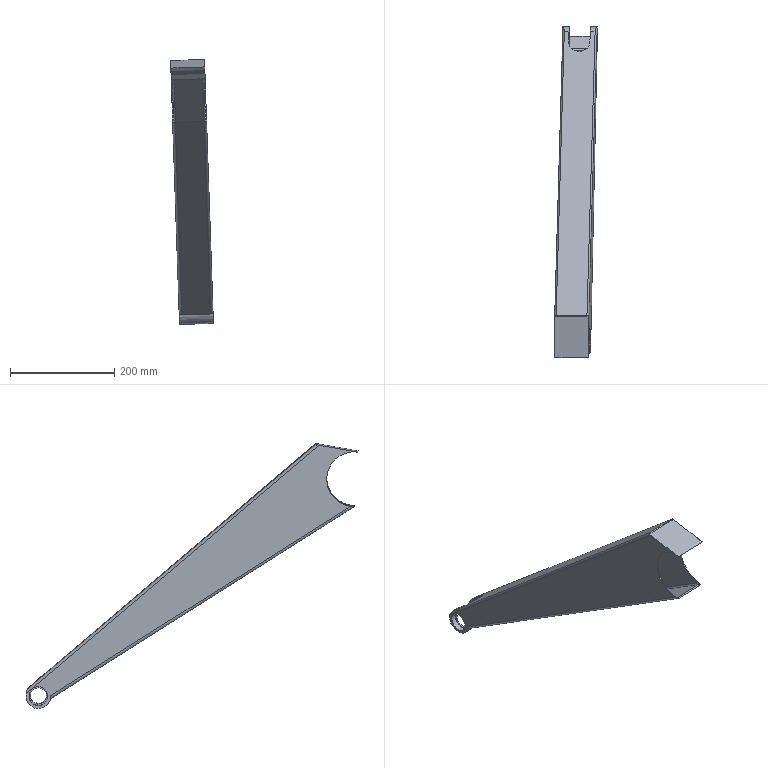Part | STEP file | 2026.6.15-Main Assembly图.sldasm-Part-134 | 1 solid | 52 faces | box 82.035 x 635.638 x 507.509 mm | volume 499419 mm3 | cylinder 29 | plane 22 | spline 1 | commonest cylinder face diameters 47.5 x8 7 x6 10 x4 31 x4 36 x4 40 x2